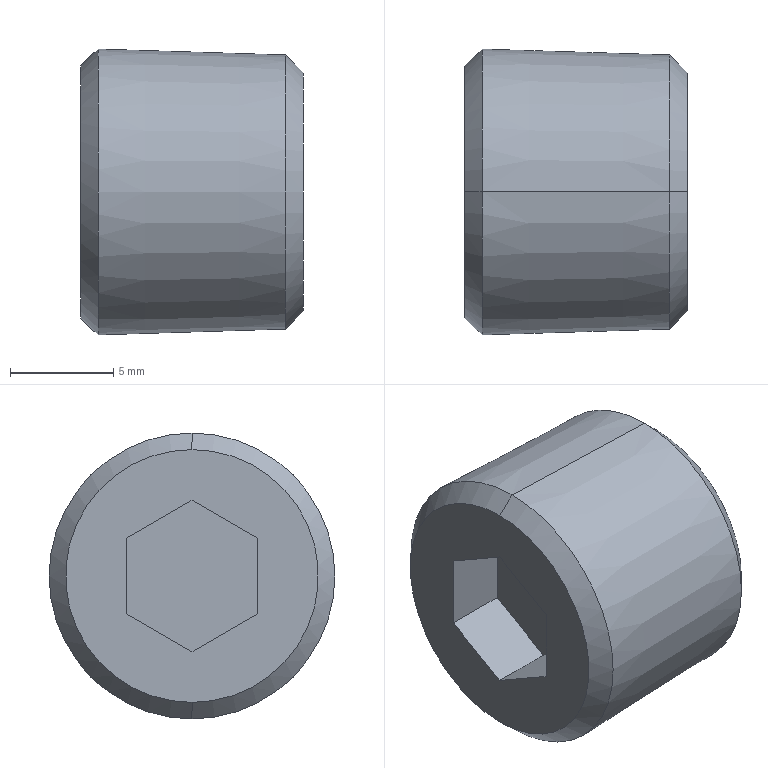Part | STEP file | AC40-04-KSTV-38JNR_AC3009A Plug | 1 solid | 15 faces | box 10.8 x 13.845 x 13.845 mm | volume 1426 mm3 | plane 9 | cone 6
STEP:
#1=CARTESIAN_POINT('',(0.,0.,0.));
#2=DIRECTION('',(0.,0.,1.));
#3=DIRECTION('',(1.,0.,0.));
#4=AXIS2_PLACEMENT_3D('',#1,#2,#3);
#5=CARTESIAN_POINT('',(0.,0.,6.124));
#6=VERTEX_POINT('',#5);
#7=CARTESIAN_POINT('',(0.,0.,-6.124));
#8=VERTEX_POINT('',#7);
#9=CARTESIAN_POINT('',(0.,0.,0.));
#10=DIRECTION('',(-1.,0.,0.));
#11=DIRECTION('',(0.,0.,-1.));
#12=AXIS2_PLACEMENT_3D('',#9,#10,#11);
#13=CIRCLE('',#12,6.124);
#14=CARTESIAN_POINT('',(0.,0.,0.));
#15=DIRECTION('',(1.,0.,0.));
#16=DIRECTION('',(0.,0.,-1.));
#17=AXIS2_PLACEMENT_3D('',#14,#15,#16);
#18=CONICAL_SURFACE('',#17,6.124,0.7543);
#19=CARTESIAN_POINT('',(6.283,0.));
#20=DIRECTION('',(-1.,0.));
#21=VECTOR('',#20,1.);
#22=LINE('',#19,#21);
#23=(GEOMETRIC_REPRESENTATION_CONTEXT(2)PARAMETRIC_REPRESENTATION_CONTEXT()REPRESENTATION_CONTEXT('',''));
#24=DEFINITIONAL_REPRESENTATION('',(#22),#23);
#25=PCURVE('',#18,#24);
#26=CARTESIAN_POINT('',(0.,0.,0.));
#27=DIRECTION('',(1.,0.,0.));
#28=DIRECTION('',(0.,0.,-1.));
#29=AXIS2_PLACEMENT_3D('',#26,#27,#28);
#30=PLANE('',#29);
#31=CARTESIAN_POINT('',(6.124,0.));
#32=CARTESIAN_POINT('',(6.124,-10.608));
#33=CARTESIAN_POINT('',(-3.062,-5.304));
#34=CARTESIAN_POINT('',(-12.249,0.));
#35=CARTESIAN_POINT('',(-3.062,5.304));
#36=CARTESIAN_POINT('',(6.124,10.608));
#37=CARTESIAN_POINT('',(6.124,0.));
#38=(BOUNDED_CURVE()B_SPLINE_CURVE(2,(#31,#32,#33,#34,#35,#36,#37),.UNSPECIFIED.,.T.,.F.)B_SPLINE_CURVE_WITH_KNOTS((1,2,2,2,2,1),(-2.094,0.,2.094,4.189,6.283,8.378),.UNSPECIFIED.)CURVE()GEOMETRIC_REPRESENTATION_ITEM()RATIONAL_B_SPLINE_CURVE((1.,0.5,1.,0.5,1.,0.5,1.))REPRESENTATION_ITEM(''));
#39=(GEOMETRIC_REPRESENTATION_CONTEXT(2)PARAMETRIC_REPRESENTATION_CONTEXT()REPRESENTATION_CONTEXT('',''));
#40=DEFINITIONAL_REPRESENTATION('',(#38),#39);
#41=PCURVE('',#30,#40);
#42=SURFACE_CURVE('',#13,(#25,#41),.PCURVE_S1.);
#43=EDGE_CURVE('',#6,#8,#42,.T.);
#44=ORIENTED_EDGE('',*,*,#43,.F.);
#45=CARTESIAN_POINT('',(0.8496,0.,6.923));
#46=VERTEX_POINT('',#45);
#47=CARTESIAN_POINT('',(0.,0.,6.124));
#48=DIRECTION('',(0.7288,0.,0.6848));
#49=VECTOR('',#48,1.);
#50=LINE('',#47,#49);
#51=CARTESIAN_POINT('',(3.142,0.));
#52=DIRECTION('',(0.,1.));
#53=VECTOR('',#52,1.);
#54=LINE('',#51,#53);
#55=(GEOMETRIC_REPRESENTATION_CONTEXT(2)PARAMETRIC_REPRESENTATION_CONTEXT()REPRESENTATION_CONTEXT('',''));
#56=DEFINITIONAL_REPRESENTATION('',(#54),#55);
#57=PCURVE('',#18,#56);
#58=CARTESIAN_POINT('',(0.,0.,0.));
#59=DIRECTION('',(1.,0.,0.));
#60=DIRECTION('',(0.,0.,-1.));
#61=AXIS2_PLACEMENT_3D('',#58,#59,#60);
#62=CONICAL_SURFACE('',#61,6.124,0.7543);
#63=CARTESIAN_POINT('',(3.142,0.));
#64=DIRECTION('',(0.,1.));
#65=VECTOR('',#64,1.);
#66=LINE('',#63,#65);
#67=(GEOMETRIC_REPRESENTATION_CONTEXT(2)PARAMETRIC_REPRESENTATION_CONTEXT()REPRESENTATION_CONTEXT('',''));
#68=DEFINITIONAL_REPRESENTATION('',(#66),#67);
#69=PCURVE('',#62,#68);
#70=SURFACE_CURVE('',#50,(#57,#69),.PCURVE_S1.);
#71=EDGE_CURVE('',#6,#46,#70,.T.);
#72=ORIENTED_EDGE('',*,*,#71,.T.);
#73=CARTESIAN_POINT('',(0.8496,0.,-6.923));
#74=VERTEX_POINT('',#73);
#75=CARTESIAN_POINT('',(0.8496,0.,0.));
#76=DIRECTION('',(1.,0.,0.));
#77=DIRECTION('',(0.,0.,-1.));
#78=AXIS2_PLACEMENT_3D('',#75,#76,#77);
#79=CIRCLE('',#78,6.923);
#80=CARTESIAN_POINT('',(0.,0.8496));
#81=DIRECTION('',(1.,0.));
#82=VECTOR('',#81,1.);
#83=LINE('',#80,#82);
#84=(GEOMETRIC_REPRESENTATION_CONTEXT(2)PARAMETRIC_REPRESENTATION_CONTEXT()REPRESENTATION_CONTEXT('',''));
#85=DEFINITIONAL_REPRESENTATION('',(#83),#84);
#86=PCURVE('',#18,#85);
#87=CARTESIAN_POINT('',(10.8,0.,0.));
#88=DIRECTION('',(-1.,0.,0.));
#89=DIRECTION('',(0.,0.,1.));
#90=AXIS2_PLACEMENT_3D('',#87,#88,#89);
#91=CONICAL_SURFACE('',#90,6.613,0.03112);
#92=CARTESIAN_POINT('',(3.142,9.95));
#93=DIRECTION('',(-1.,0.));
#94=VECTOR('',#93,1.);
#95=LINE('',#92,#94);
#96=(GEOMETRIC_REPRESENTATION_CONTEXT(2)PARAMETRIC_REPRESENTATION_CONTEXT()REPRESENTATION_CONTEXT('',''));
#97=DEFINITIONAL_REPRESENTATION('',(#95),#96);
#98=PCURVE('',#91,#97);
#99=SURFACE_CURVE('',#79,(#86,#98),.PCURVE_S1.);
#100=EDGE_CURVE('',#74,#46,#99,.T.);
#101=ORIENTED_EDGE('',*,*,#100,.F.);
#102=CARTESIAN_POINT('',(0.,0.,-6.124));
#103=DIRECTION('',(0.7288,0.,-0.6848));
#104=VECTOR('',#103,1.);
#105=LINE('',#102,#104);
#106=CARTESIAN_POINT('',(0.,0.));
#107=DIRECTION('',(0.,1.));
#108=VECTOR('',#107,1.);
#109=LINE('',#106,#108);
#110=(GEOMETRIC_REPRESENTATION_CONTEXT(2)PARAMETRIC_REPRESENTATION_CONTEXT()REPRESENTATION_CONTEXT('',''));
#111=DEFINITIONAL_REPRESENTATION('',(#109),#110);
#112=PCURVE('',#18,#111);
#113=CARTESIAN_POINT('',(6.283,0.));
#114=DIRECTION('',(0.,1.));
#115=VECTOR('',#114,1.);
#116=LINE('',#113,#115);
#117=(GEOMETRIC_REPRESENTATION_CONTEXT(2)PARAMETRIC_REPRESENTATION_CONTEXT()REPRESENTATION_CONTEXT('',''));
#118=DEFINITIONAL_REPRESENTATION('',(#116),#117);
#119=PCURVE('',#62,#118);
#120=SURFACE_CURVE('',#105,(#112,#119),.PCURVE_S1.);
#121=EDGE_CURVE('',#8,#74,#120,.T.);
#122=ORIENTED_EDGE('',*,*,#121,.F.);
#123=EDGE_LOOP('',(#44,#72,#101,#122));
#124=FACE_BOUND('',#123,.T.);
#125=ADVANCED_FACE('',(#124),#18,.T.);
#126=CARTESIAN_POINT('',(10.8,0.,-5.763));
#127=VERTEX_POINT('',#126);
#128=CARTESIAN_POINT('',(10.8,0.,5.763));
#129=VERTEX_POINT('',#128);
#130=CARTESIAN_POINT('',(10.8,0.,0.));
#131=DIRECTION('',(1.,0.,0.));
#132=DIRECTION('',(0.,0.,1.));
#133=AXIS2_PLACEMENT_3D('',#130,#131,#132);
#134=CIRCLE('',#133,5.763);
#135=CARTESIAN_POINT('',(9.923,0.,0.));
#136=DIRECTION('',(-1.,0.,0.));
#137=DIRECTION('',(0.,0.,1.));
#138=AXIS2_PLACEMENT_3D('',#135,#136,#137);
#139=CONICAL_SURFACE('',#138,6.64,0.7854);
#140=CARTESIAN_POINT('',(6.283,-0.8773));
#141=DIRECTION('',(-1.,0.));
#142=VECTOR('',#141,1.);
#143=LINE('',#140,#142);
#144=(GEOMETRIC_REPRESENTATION_CONTEXT(2)PARAMETRIC_REPRESENTATION_CONTEXT()REPRESENTATION_CONTEXT('',''));
#145=DEFINITIONAL_REPRESENTATION('',(#143),#144);
#146=PCURVE('',#139,#145);
#147=CARTESIAN_POINT('',(10.8,6.613,0.));
#148=DIRECTION('',(-1.,0.,0.));
#149=DIRECTION('',(0.,0.,1.));
#150=AXIS2_PLACEMENT_3D('',#147,#148,#149);
#151=PLANE('',#150);
#152=CARTESIAN_POINT('',(5.763,-6.613));
#153=CARTESIAN_POINT('',(5.763,-16.595));
#154=CARTESIAN_POINT('',(-2.881,-11.604));
#155=CARTESIAN_POINT('',(-11.526,-6.613));
#156=CARTESIAN_POINT('',(-2.881,-1.622));
#157=CARTESIAN_POINT('',(5.763,3.369));
#158=CARTESIAN_POINT('',(5.763,-6.613));
#159=(BOUNDED_CURVE()B_SPLINE_CURVE(2,(#152,#153,#154,#155,#156,#157,#158),.UNSPECIFIED.,.T.,.F.)B_SPLINE_CURVE_WITH_KNOTS((1,2,2,2,2,1),(-2.094,0.,2.094,4.189,6.283,8.378),.UNSPECIFIED.)CURVE()GEOMETRIC_REPRESENTATION_ITEM()RATIONAL_B_SPLINE_CURVE((1.,0.5,1.,0.5,1.,0.5,1.))REPRESENTATION_ITEM(''));
#160=(GEOMETRIC_REPRESENTATION_CONTEXT(2)PARAMETRIC_REPRESENTATION_CONTEXT()REPRESENTATION_CONTEXT('',''));
#161=DEFINITIONAL_REPRESENTATION('',(#159),#160);
#162=PCURVE('',#151,#161);
#163=SURFACE_CURVE('',#134,(#146,#162),.PCURVE_S1.);
#164=EDGE_CURVE('',#127,#129,#163,.T.);
#165=ORIENTED_EDGE('',*,*,#164,.F.);
#166=CARTESIAN_POINT('',(9.923,0.,-6.64));
#167=VERTEX_POINT('',#166);
#168=CARTESIAN_POINT('',(9.923,0.,-6.64));
#169=DIRECTION('',(-0.7071,0.,-0.7071));
#170=VECTOR('',#169,1.);
#171=LINE('',#168,#170);
#172=CARTESIAN_POINT('',(3.142,0.));
#173=DIRECTION('',(0.,1.));
#174=VECTOR('',#173,1.);
#175=LINE('',#172,#174);
#176=(GEOMETRIC_REPRESENTATION_CONTEXT(2)PARAMETRIC_REPRESENTATION_CONTEXT()REPRESENTATION_CONTEXT('',''));
#177=DEFINITIONAL_REPRESENTATION('',(#175),#176);
#178=PCURVE('',#139,#177);
#179=CARTESIAN_POINT('',(9.923,0.,0.));
#180=DIRECTION('',(-1.,0.,0.));
#181=DIRECTION('',(0.,0.,1.));
#182=AXIS2_PLACEMENT_3D('',#179,#180,#181);
#183=CONICAL_SURFACE('',#182,6.64,0.7854);
#184=CARTESIAN_POINT('',(3.142,0.));
#185=DIRECTION('',(0.,1.));
#186=VECTOR('',#185,1.);
#187=LINE('',#184,#186);
#188=(GEOMETRIC_REPRESENTATION_CONTEXT(2)PARAMETRIC_REPRESENTATION_CONTEXT()REPRESENTATION_CONTEXT('',''));
#189=DEFINITIONAL_REPRESENTATION('',(#187),#188);
#190=PCURVE('',#183,#189);
#191=SURFACE_CURVE('',#171,(#178,#190),.PCURVE_S1.);
#192=EDGE_CURVE('',#127,#167,#191,.T.);
#193=ORIENTED_EDGE('',*,*,#192,.T.);
#194=CARTESIAN_POINT('',(9.923,0.,6.64));
#195=VERTEX_POINT('',#194);
#196=CARTESIAN_POINT('',(9.923,0.,0.));
#197=DIRECTION('',(-1.,0.,0.));
#198=DIRECTION('',(0.,0.,-1.));
#199=AXIS2_PLACEMENT_3D('',#196,#197,#198);
#200=CIRCLE('',#199,6.64);
#201=CARTESIAN_POINT('',(-3.142,0.));
#202=DIRECTION('',(1.,0.));
#203=VECTOR('',#202,1.);
#204=LINE('',#201,#203);
#205=(GEOMETRIC_REPRESENTATION_CONTEXT(2)PARAMETRIC_REPRESENTATION_CONTEXT()REPRESENTATION_CONTEXT('',''));
#206=DEFINITIONAL_REPRESENTATION('',(#204),#205);
#207=PCURVE('',#139,#206);
#208=CARTESIAN_POINT('',(-3.142,0.8773));
#209=DIRECTION('',(1.,0.));
#210=VECTOR('',#209,1.);
#211=LINE('',#208,#210);
#212=(GEOMETRIC_REPRESENTATION_CONTEXT(2)PARAMETRIC_REPRESENTATION_CONTEXT()REPRESENTATION_CONTEXT('',''));
#213=DEFINITIONAL_REPRESENTATION('',(#211),#212);
#214=PCURVE('',#91,#213);
#215=SURFACE_CURVE('',#200,(#207,#214),.PCURVE_S1.);
#216=EDGE_CURVE('',#195,#167,#215,.T.);
#217=ORIENTED_EDGE('',*,*,#216,.F.);
#218=CARTESIAN_POINT('',(9.923,0.,6.64));
#219=DIRECTION('',(-0.7071,0.,0.7071));
#220=VECTOR('',#219,1.);
#221=LINE('',#218,#220);
#222=CARTESIAN_POINT('',(0.,0.));
#223=DIRECTION('',(0.,1.));
#224=VECTOR('',#223,1.);
#225=LINE('',#222,#224);
#226=(GEOMETRIC_REPRESENTATION_CONTEXT(2)PARAMETRIC_REPRESENTATION_CONTEXT()REPRESENTATION_CONTEXT('',''));
#227=DEFINITIONAL_REPRESENTATION('',(#225),#226);
#228=PCURVE('',#139,#227);
#229=CARTESIAN_POINT('',(6.283,0.));
#230=DIRECTION('',(0.,1.));
#231=VECTOR('',#230,1.);
#232=LINE('',#229,#231);
#233=(GEOMETRIC_REPRESENTATION_CONTEXT(2)PARAMETRIC_REPRESENTATION_CONTEXT()REPRESENTATION_CONTEXT('',''));
#234=DEFINITIONAL_REPRESENTATION('',(#232),#233);
#235=PCURVE('',#183,#234);
#236=SURFACE_CURVE('',#221,(#228,#235),.PCURVE_S1.);
#237=EDGE_CURVE('',#129,#195,#236,.T.);
#238=ORIENTED_EDGE('',*,*,#237,.F.);
#239=EDGE_LOOP('',(#165,#193,#217,#238));
#240=FACE_BOUND('',#239,.T.);
#241=ADVANCED_FACE('',(#240),#139,.T.);
#242=ORIENTED_EDGE('',*,*,#216,.T.);
#243=CARTESIAN_POINT('',(10.8,0.,-6.613));
#244=DIRECTION('',(-0.9995,0.,-0.03111));
#245=VECTOR('',#244,1.);
#246=LINE('',#243,#245);
#247=CARTESIAN_POINT('',(3.142,0.));
#248=DIRECTION('',(0.,1.));
#249=VECTOR('',#248,1.);
#250=LINE('',#247,#249);
#251=(GEOMETRIC_REPRESENTATION_CONTEXT(2)PARAMETRIC_REPRESENTATION_CONTEXT()REPRESENTATION_CONTEXT('',''));
#252=DEFINITIONAL_REPRESENTATION('',(#250),#251);
#253=PCURVE('',#91,#252);
#254=CARTESIAN_POINT('',(10.8,0.,0.));
#255=DIRECTION('',(-1.,0.,0.));
#256=DIRECTION('',(0.,0.,1.));
#257=AXIS2_PLACEMENT_3D('',#254,#255,#256);
#258=CONICAL_SURFACE('',#257,6.613,0.03112);
#259=CARTESIAN_POINT('',(3.142,0.));
#260=DIRECTION('',(0.,1.));
#261=VECTOR('',#260,1.);
#262=LINE('',#259,#261);
#263=(GEOMETRIC_REPRESENTATION_CONTEXT(2)PARAMETRIC_REPRESENTATION_CONTEXT()REPRESENTATION_CONTEXT('',''));
#264=DEFINITIONAL_REPRESENTATION('',(#262),#263);
#265=PCURVE('',#258,#264);
#266=SURFACE_CURVE('',#246,(#253,#265),.PCURVE_S1.);
#267=EDGE_CURVE('',#167,#74,#266,.T.);
#268=ORIENTED_EDGE('',*,*,#267,.T.);
#269=ORIENTED_EDGE('',*,*,#100,.T.);
#270=CARTESIAN_POINT('',(10.8,0.,6.613));
#271=DIRECTION('',(-0.9995,0.,0.03111));
#272=VECTOR('',#271,1.);
#273=LINE('',#270,#272);
#274=CARTESIAN_POINT('',(0.,0.));
#275=DIRECTION('',(0.,1.));
#276=VECTOR('',#275,1.);
#277=LINE('',#274,#276);
#278=(GEOMETRIC_REPRESENTATION_CONTEXT(2)PARAMETRIC_REPRESENTATION_CONTEXT()REPRESENTATION_CONTEXT('',''));
#279=DEFINITIONAL_REPRESENTATION('',(#277),#278);
#280=PCURVE('',#91,#279);
#281=CARTESIAN_POINT('',(6.283,0.));
#282=DIRECTION('',(0.,1.));
#283=VECTOR('',#282,1.);
#284=LINE('',#281,#283);
#285=(GEOMETRIC_REPRESENTATION_CONTEXT(2)PARAMETRIC_REPRESENTATION_CONTEXT()REPRESENTATION_CONTEXT('',''));
#286=DEFINITIONAL_REPRESENTATION('',(#284),#285);
#287=PCURVE('',#258,#286);
#288=SURFACE_CURVE('',#273,(#280,#287),.PCURVE_S1.);
#289=EDGE_CURVE('',#195,#46,#288,.T.);
#290=ORIENTED_EDGE('',*,*,#289,.F.);
#291=EDGE_LOOP('',(#242,#268,#269,#290));
#292=FACE_BOUND('',#291,.T.);
#293=ADVANCED_FACE('',(#292),#91,.T.);
#294=CARTESIAN_POINT('',(10.8,0.,0.));
#295=DIRECTION('',(1.,0.,0.));
#296=DIRECTION('',(0.,0.,1.));
#297=AXIS2_PLACEMENT_3D('',#294,#295,#296);
#298=CIRCLE('',#297,5.763);
#299=CARTESIAN_POINT('',(5.763,-6.613));
#300=CARTESIAN_POINT('',(5.763,-16.595));
#301=CARTESIAN_POINT('',(-2.881,-11.604));
#302=CARTESIAN_POINT('',(-11.526,-6.613));
#303=CARTESIAN_POINT('',(-2.881,-1.622));
#304=CARTESIAN_POINT('',(5.763,3.369));
#305=CARTESIAN_POINT('',(5.763,-6.613));
#306=(BOUNDED_CURVE()B_SPLINE_CURVE(2,(#299,#300,#301,#302,#303,#304,#305),.UNSPECIFIED.,.T.,.F.)B_SPLINE_CURVE_WITH_KNOTS((1,2,2,2,2,1),(-2.094,0.,2.094,4.189,6.283,8.378),.UNSPECIFIED.)CURVE()GEOMETRIC_REPRESENTATION_ITEM()RATIONAL_B_SPLINE_CURVE((1.,0.5,1.,0.5,1.,0.5,1.))REPRESENTATION_ITEM(''));
#307=(GEOMETRIC_REPRESENTATION_CONTEXT(2)PARAMETRIC_REPRESENTATION_CONTEXT()REPRESENTATION_CONTEXT('',''));
#308=DEFINITIONAL_REPRESENTATION('',(#306),#307);
#309=PCURVE('',#151,#308);
#310=CARTESIAN_POINT('',(6.283,-0.8773));
#311=DIRECTION('',(-1.,0.));
#312=VECTOR('',#311,1.);
#313=LINE('',#310,#312);
#314=(GEOMETRIC_REPRESENTATION_CONTEXT(2)PARAMETRIC_REPRESENTATION_CONTEXT()REPRESENTATION_CONTEXT('',''));
#315=DEFINITIONAL_REPRESENTATION('',(#313),#314);
#316=PCURVE('',#183,#315);
#317=SURFACE_CURVE('',#298,(#309,#316),.PCURVE_S1.);
#318=EDGE_CURVE('',#129,#127,#317,.T.);
#319=ORIENTED_EDGE('',*,*,#318,.T.);
#320=ORIENTED_EDGE('',*,*,#164,.T.);
#321=EDGE_LOOP('',(#319,#320));
#322=FACE_BOUND('',#321,.T.);
#323=ADVANCED_FACE('',(#322),#151,.F.);
#324=ORIENTED_EDGE('',*,*,#267,.F.);
#325=CARTESIAN_POINT('',(9.923,0.,0.));
#326=DIRECTION('',(-1.,0.,0.));
#327=DIRECTION('',(0.,0.,-1.));
#328=AXIS2_PLACEMENT_3D('',#325,#326,#327);
#329=CIRCLE('',#328,6.64);
#330=CARTESIAN_POINT('',(3.142,0.8773));
#331=DIRECTION('',(1.,0.));
#332=VECTOR('',#331,1.);
#333=LINE('',#330,#332);
#334=(GEOMETRIC_REPRESENTATION_CONTEXT(2)PARAMETRIC_REPRESENTATION_CONTEXT()REPRESENTATION_CONTEXT('',''));
#335=DEFINITIONAL_REPRESENTATION('',(#333),#334);
#336=PCURVE('',#258,#335);
#337=CARTESIAN_POINT('',(3.142,0.));
#338=DIRECTION('',(1.,0.));
#339=VECTOR('',#338,1.);
#340=LINE('',#337,#339);
#341=(GEOMETRIC_REPRESENTATION_CONTEXT(2)PARAMETRIC_REPRESENTATION_CONTEXT()REPRESENTATION_CONTEXT('',''));
#342=DEFINITIONAL_REPRESENTATION('',(#340),#341);
#343=PCURVE('',#183,#342);
#344=SURFACE_CURVE('',#329,(#336,#343),.PCURVE_S1.);
#345=EDGE_CURVE('',#167,#195,#344,.T.);
#346=ORIENTED_EDGE('',*,*,#345,.T.);
#347=ORIENTED_EDGE('',*,*,#289,.T.);
#348=CARTESIAN_POINT('',(0.8496,0.,0.));
#349=DIRECTION('',(1.,0.,0.));
#350=DIRECTION('',(0.,0.,-1.));
#351=AXIS2_PLACEMENT_3D('',#348,#349,#350);
#352=CIRCLE('',#351,6.923);
#353=CARTESIAN_POINT('',(9.425,9.95));
#354=DIRECTION('',(-1.,0.));
#355=VECTOR('',#354,1.);
#356=LINE('',#353,#355);
#357=(GEOMETRIC_REPRESENTATION_CONTEXT(2)PARAMETRIC_REPRESENTATION_CONTEXT()REPRESENTATION_CONTEXT('',''));
#358=DEFINITIONAL_REPRESENTATION('',(#356),#357);
#359=PCURVE('',#258,#358);
#360=CARTESIAN_POINT('',(0.,0.8496));
#361=DIRECTION('',(1.,0.));
#362=VECTOR('',#361,1.);
#363=LINE('',#360,#362);
#364=(GEOMETRIC_REPRESENTATION_CONTEXT(2)PARAMETRIC_REPRESENTATION_CONTEXT()REPRESENTATION_CONTEXT('',''));
#365=DEFINITIONAL_REPRESENTATION('',(#363),#364);
#366=PCURVE('',#62,#365);
#367=SURFACE_CURVE('',#352,(#359,#366),.PCURVE_S1.);
#368=EDGE_CURVE('',#46,#74,#367,.T.);
#369=ORIENTED_EDGE('',*,*,#368,.T.);
#370=EDGE_LOOP('',(#324,#346,#347,#369));
#371=FACE_BOUND('',#370,.T.);
#372=ADVANCED_FACE('',(#371),#258,.T.);
#373=CARTESIAN_POINT('',(0.,0.,3.666));
#374=VERTEX_POINT('',#373);
#375=CARTESIAN_POINT('',(0.,3.175,1.833));
#376=VERTEX_POINT('',#375);
#377=CARTESIAN_POINT('',(0.,0.,3.666));
#378=DIRECTION('',(0.,0.866,-0.5));
#379=VECTOR('',#378,1.);
#380=LINE('',#377,#379);
#381=CARTESIAN_POINT('',(-3.666,0.));
#382=DIRECTION('',(0.5,0.866));
#383=VECTOR('',#382,1.);
#384=LINE('',#381,#383);
#385=(GEOMETRIC_REPRESENTATION_CONTEXT(2)PARAMETRIC_REPRESENTATION_CONTEXT()REPRESENTATION_CONTEXT('',''));
#386=DEFINITIONAL_REPRESENTATION('',(#384),#385);
#387=PCURVE('',#30,#386);
#388=CARTESIAN_POINT('',(3.,0.,3.666));
#389=DIRECTION('',(0.,0.5,0.866));
#390=DIRECTION('',(0.,-0.866,0.5));
#391=AXIS2_PLACEMENT_3D('',#388,#389,#390);
#392=PLANE('',#391);
#393=CARTESIAN_POINT('',(0.,-3.));
#394=DIRECTION('',(-1.,0.));
#395=VECTOR('',#394,1.);
#396=LINE('',#393,#395);
#397=(GEOMETRIC_REPRESENTATION_CONTEXT(2)PARAMETRIC_REPRESENTATION_CONTEXT()REPRESENTATION_CONTEXT('',''));
#398=DEFINITIONAL_REPRESENTATION('',(#396),#397);
#399=PCURVE('',#392,#398);
#400=SURFACE_CURVE('',#380,(#387,#399),.PCURVE_S1.);
#401=EDGE_CURVE('',#374,#376,#400,.T.);
#402=ORIENTED_EDGE('',*,*,#401,.F.);
#403=CARTESIAN_POINT('',(0.,-3.175,1.833));
#404=VERTEX_POINT('',#403);
#405=CARTESIAN_POINT('',(0.,-3.175,1.833));
#406=DIRECTION('',(0.,0.866,0.5));
#407=VECTOR('',#406,1.);
#408=LINE('',#405,#407);
#409=CARTESIAN_POINT('',(-1.833,-3.175));
#410=DIRECTION('',(-0.5,0.866));
#411=VECTOR('',#410,1.);
#412=LINE('',#409,#411);
#413=(GEOMETRIC_REPRESENTATION_CONTEXT(2)PARAMETRIC_REPRESENTATION_CONTEXT()REPRESENTATION_CONTEXT('',''));
#414=DEFINITIONAL_REPRESENTATION('',(#412),#413);
#415=PCURVE('',#30,#414);
#416=CARTESIAN_POINT('',(3.,-3.175,1.833));
#417=DIRECTION('',(0.,-0.5,0.866));
#418=DIRECTION('',(0.,-0.866,-0.5));
#419=AXIS2_PLACEMENT_3D('',#416,#417,#418);
#420=PLANE('',#419);
#421=CARTESIAN_POINT('',(0.,-3.));
#422=DIRECTION('',(-1.,0.));
#423=VECTOR('',#422,1.);
#424=LINE('',#421,#423);
#425=(GEOMETRIC_REPRESENTATION_CONTEXT(2)PARAMETRIC_REPRESENTATION_CONTEXT()REPRESENTATION_CONTEXT('',''));
#426=DEFINITIONAL_REPRESENTATION('',(#424),#425);
#427=PCURVE('',#420,#426);
#428=SURFACE_CURVE('',#408,(#415,#427),.PCURVE_S1.);
#429=EDGE_CURVE('',#404,#374,#428,.T.);
#430=ORIENTED_EDGE('',*,*,#429,.F.);
#431=CARTESIAN_POINT('',(0.,-3.175,-1.833));
#432=VERTEX_POINT('',#431);
#433=CARTESIAN_POINT('',(0.,-3.175,-1.833));
#434=DIRECTION('',(0.,0.,1.));
#435=VECTOR('',#434,1.);
#436=LINE('',#433,#435);
#437=CARTESIAN_POINT('',(1.833,-3.175));
#438=DIRECTION('',(-1.,0.));
#439=VECTOR('',#438,1.);
#440=LINE('',#437,#439);
#441=(GEOMETRIC_REPRESENTATION_CONTEXT(2)PARAMETRIC_REPRESENTATION_CONTEXT()REPRESENTATION_CONTEXT('',''));
#442=DEFINITIONAL_REPRESENTATION('',(#440),#441);
#443=PCURVE('',#30,#442);
#444=CARTESIAN_POINT('',(3.,-3.175,-1.833));
#445=DIRECTION('',(0.,-1.,0.));
#446=DIRECTION('',(0.,0.,-1.));
#447=AXIS2_PLACEMENT_3D('',#444,#445,#446);
#448=PLANE('',#447);
#449=CARTESIAN_POINT('',(0.,-3.));
#450=DIRECTION('',(-1.,0.));
#451=VECTOR('',#450,1.);
#452=LINE('',#449,#451);
#453=(GEOMETRIC_REPRESENTATION_CONTEXT(2)PARAMETRIC_REPRESENTATION_CONTEXT()REPRESENTATION_CONTEXT('',''));
#454=DEFINITIONAL_REPRESENTATION('',(#452),#453);
#455=PCURVE('',#448,#454);
#456=SURFACE_CURVE('',#436,(#443,#455),.PCURVE_S1.);
#457=EDGE_CURVE('',#432,#404,#456,.T.);
#458=ORIENTED_EDGE('',*,*,#457,.F.);
#459=CARTESIAN_POINT('',(0.,0.,-3.666));
#460=VERTEX_POINT('',#459);
#461=CARTESIAN_POINT('',(0.,0.,-3.666));
#462=DIRECTION('',(0.,-0.866,0.5));
#463=VECTOR('',#462,1.);
#464=LINE('',#461,#463);
#465=CARTESIAN_POINT('',(3.666,0.));
#466=DIRECTION('',(-0.5,-0.866));
#467=VECTOR('',#466,1.);
#468=LINE('',#465,#467);
#469=(GEOMETRIC_REPRESENTATION_CONTEXT(2)PARAMETRIC_REPRESENTATION_CONTEXT()REPRESENTATION_CONTEXT('',''));
#470=DEFINITIONAL_REPRESENTATION('',(#468),#469);
#471=PCURVE('',#30,#470);
#472=CARTESIAN_POINT('',(3.,0.,-3.666));
#473=DIRECTION('',(0.,-0.5,-0.866));
#474=DIRECTION('',(0.,0.866,-0.5));
#475=AXIS2_PLACEMENT_3D('',#472,#473,#474);
#476=PLANE('',#475);
#477=CARTESIAN_POINT('',(0.,-3.));
#478=DIRECTION('',(-1.,0.));
#479=VECTOR('',#478,1.);
#480=LINE('',#477,#479);
#481=(GEOMETRIC_REPRESENTATION_CONTEXT(2)PARAMETRIC_REPRESENTATION_CONTEXT()REPRESENTATION_CONTEXT('',''));
#482=DEFINITIONAL_REPRESENTATION('',(#480),#481);
#483=PCURVE('',#476,#482);
#484=SURFACE_CURVE('',#464,(#471,#483),.PCURVE_S1.);
#485=EDGE_CURVE('',#460,#432,#484,.T.);
#486=ORIENTED_EDGE('',*,*,#485,.F.);
#487=CARTESIAN_POINT('',(0.,3.175,-1.833));
#488=VERTEX_POINT('',#487);
#489=CARTESIAN_POINT('',(0.,3.175,-1.833));
#490=DIRECTION('',(0.,-0.866,-0.5));
#491=VECTOR('',#490,1.);
#492=LINE('',#489,#491);
#493=CARTESIAN_POINT('',(1.833,3.175));
#494=DIRECTION('',(0.5,-0.866));
#495=VECTOR('',#494,1.);
#496=LINE('',#493,#495);
#497=(GEOMETRIC_REPRESENTATION_CONTEXT(2)PARAMETRIC_REPRESENTATION_CONTEXT()REPRESENTATION_CONTEXT('',''));
#498=DEFINITIONAL_REPRESENTATION('',(#496),#497);
#499=PCURVE('',#30,#498);
#500=CARTESIAN_POINT('',(3.,3.175,-1.833));
#501=DIRECTION('',(0.,0.5,-0.866));
#502=DIRECTION('',(0.,0.866,0.5));
#503=AXIS2_PLACEMENT_3D('',#500,#501,#502);
#504=PLANE('',#503);
#505=CARTESIAN_POINT('',(0.,-3.));
#506=DIRECTION('',(-1.,0.));
#507=VECTOR('',#506,1.);
#508=LINE('',#505,#507);
#509=(GEOMETRIC_REPRESENTATION_CONTEXT(2)PARAMETRIC_REPRESENTATION_CONTEXT()REPRESENTATION_CONTEXT('',''));
#510=DEFINITIONAL_REPRESENTATION('',(#508),#509);
#511=PCURVE('',#504,#510);
#512=SURFACE_CURVE('',#492,(#499,#511),.PCURVE_S1.);
#513=EDGE_CURVE('',#488,#460,#512,.T.);
#514=ORIENTED_EDGE('',*,*,#513,.F.);
#515=CARTESIAN_POINT('',(0.,3.175,1.833));
#516=DIRECTION('',(0.,0.,-1.));
#517=VECTOR('',#516,1.);
#518=LINE('',#515,#517);
#519=CARTESIAN_POINT('',(-1.833,3.175));
#520=DIRECTION('',(1.,0.));
#521=VECTOR('',#520,1.);
#522=LINE('',#519,#521);
#523=(GEOMETRIC_REPRESENTATION_CONTEXT(2)PARAMETRIC_REPRESENTATION_CONTEXT()REPRESENTATION_CONTEXT('',''));
#524=DEFINITIONAL_REPRESENTATION('',(#522),#523);
#525=PCURVE('',#30,#524);
#526=CARTESIAN_POINT('',(3.,3.175,1.833));
#527=DIRECTION('',(0.,1.,0.));
#528=DIRECTION('',(0.,0.,1.));
#529=AXIS2_PLACEMENT_3D('',#526,#527,#528);
#530=PLANE('',#529);
#531=CARTESIAN_POINT('',(0.,-3.));
#532=DIRECTION('',(-1.,0.));
#533=VECTOR('',#532,1.);
#534=LINE('',#531,#533);
#535=(GEOMETRIC_REPRESENTATION_CONTEXT(2)PARAMETRIC_REPRESENTATION_CONTEXT()REPRESENTATION_CONTEXT('',''));
#536=DEFINITIONAL_REPRESENTATION('',(#534),#535);
#537=PCURVE('',#530,#536);
#538=SURFACE_CURVE('',#518,(#525,#537),.PCURVE_S1.);
#539=EDGE_CURVE('',#376,#488,#538,.T.);
#540=ORIENTED_EDGE('',*,*,#539,.F.);
#541=EDGE_LOOP('',(#402,#430,#458,#486,#514,#540));
#542=FACE_BOUND('',#541,.T.);
#543=CARTESIAN_POINT('',(0.,0.,0.));
#544=DIRECTION('',(-1.,0.,0.));
#545=DIRECTION('',(0.,0.,-1.));
#546=AXIS2_PLACEMENT_3D('',#543,#544,#545);
#547=CIRCLE('',#546,6.124);
#548=CARTESIAN_POINT('',(6.124,0.));
#549=CARTESIAN_POINT('',(6.124,-10.608));
#550=CARTESIAN_POINT('',(-3.062,-5.304));
#551=CARTESIAN_POINT('',(-12.249,0.));
#552=CARTESIAN_POINT('',(-3.062,5.304));
#553=CARTESIAN_POINT('',(6.124,10.608));
#554=CARTESIAN_POINT('',(6.124,0.));
#555=(BOUNDED_CURVE()B_SPLINE_CURVE(2,(#548,#549,#550,#551,#552,#553,#554),.UNSPECIFIED.,.T.,.F.)B_SPLINE_CURVE_WITH_KNOTS((1,2,2,2,2,1),(-2.094,0.,2.094,4.189,6.283,8.378),.UNSPECIFIED.)CURVE()GEOMETRIC_REPRESENTATION_ITEM()RATIONAL_B_SPLINE_CURVE((1.,0.5,1.,0.5,1.,0.5,1.))REPRESENTATION_ITEM(''));
#556=(GEOMETRIC_REPRESENTATION_CONTEXT(2)PARAMETRIC_REPRESENTATION_CONTEXT()REPRESENTATION_CONTEXT('',''));
#557=DEFINITIONAL_REPRESENTATION('',(#555),#556);
#558=PCURVE('',#30,#557);
#559=CARTESIAN_POINT('',(6.283,0.));
#560=DIRECTION('',(-1.,0.));
#561=VECTOR('',#560,1.);
#562=LINE('',#559,#561);
#563=(GEOMETRIC_REPRESENTATION_CONTEXT(2)PARAMETRIC_REPRESENTATION_CONTEXT()REPRESENTATION_CONTEXT('',''));
#564=DEFINITIONAL_REPRESENTATION('',(#562),#563);
#565=PCURVE('',#62,#564);
#566=SURFACE_CURVE('',#547,(#558,#565),.PCURVE_S1.);
#567=EDGE_CURVE('',#8,#6,#566,.T.);
#568=ORIENTED_EDGE('',*,*,#567,.T.);
#569=ORIENTED_EDGE('',*,*,#43,.T.);
#570=EDGE_LOOP('',(#568,#569));
#571=FACE_BOUND('',#570,.T.);
#572=ADVANCED_FACE('',(#542,#571),#30,.F.);
#573=ORIENTED_EDGE('',*,*,#192,.F.);
#574=ORIENTED_EDGE('',*,*,#318,.F.);
#575=ORIENTED_EDGE('',*,*,#237,.T.);
#576=ORIENTED_EDGE('',*,*,#345,.F.);
#577=EDGE_LOOP('',(#573,#574,#575,#576));
#578=FACE_BOUND('',#577,.T.);
#579=ADVANCED_FACE('',(#578),#183,.T.);
#580=ORIENTED_EDGE('',*,*,#71,.F.);
#581=ORIENTED_EDGE('',*,*,#567,.F.);
#582=ORIENTED_EDGE('',*,*,#121,.T.);
#583=ORIENTED_EDGE('',*,*,#368,.F.);
#584=EDGE_LOOP('',(#580,#581,#582,#583));
#585=FACE_BOUND('',#584,.T.);
#586=ADVANCED_FACE('',(#585),#62,.T.);
#587=ORIENTED_EDGE('',*,*,#429,.T.);
#588=CARTESIAN_POINT('',(3.,0.,3.666));
#589=VERTEX_POINT('',#588);
#590=CARTESIAN_POINT('',(3.,0.,3.666));
#591=DIRECTION('',(-1.,0.,0.));
#592=VECTOR('',#591,1.);
#593=LINE('',#590,#592);
#594=CARTESIAN_POINT('',(-3.666,0.));
#595=DIRECTION('',(0.,-1.));
#596=VECTOR('',#595,1.);
#597=LINE('',#594,#596);
#598=(GEOMETRIC_REPRESENTATION_CONTEXT(2)PARAMETRIC_REPRESENTATION_CONTEXT()REPRESENTATION_CONTEXT('',''));
#599=DEFINITIONAL_REPRESENTATION('',(#597),#598);
#600=PCURVE('',#420,#599);
#601=CARTESIAN_POINT('',(0.,0.));
#602=DIRECTION('',(0.,-1.));
#603=VECTOR('',#602,1.);
#604=LINE('',#601,#603);
#605=(GEOMETRIC_REPRESENTATION_CONTEXT(2)PARAMETRIC_REPRESENTATION_CONTEXT()REPRESENTATION_CONTEXT('',''));
#606=DEFINITIONAL_REPRESENTATION('',(#604),#605);
#607=PCURVE('',#392,#606);
#608=SURFACE_CURVE('',#593,(#600,#607),.PCURVE_S1.);
#609=EDGE_CURVE('',#589,#374,#608,.T.);
#610=ORIENTED_EDGE('',*,*,#609,.F.);
#611=CARTESIAN_POINT('',(3.,-3.175,1.833));
#612=VERTEX_POINT('',#611);
#613=CARTESIAN_POINT('',(3.,-3.175,1.833));
#614=DIRECTION('',(0.,0.866,0.5));
#615=VECTOR('',#614,1.);
#616=LINE('',#613,#615);
#617=CARTESIAN_POINT('',(0.,0.));
#618=DIRECTION('',(-1.,0.));
#619=VECTOR('',#618,1.);
#620=LINE('',#617,#619);
#621=(GEOMETRIC_REPRESENTATION_CONTEXT(2)PARAMETRIC_REPRESENTATION_CONTEXT()REPRESENTATION_CONTEXT('',''));
#622=DEFINITIONAL_REPRESENTATION('',(#620),#621);
#623=PCURVE('',#420,#622);
#624=CARTESIAN_POINT('',(3.,3.175,5.499));
#625=DIRECTION('',(-1.,0.,0.));
#626=DIRECTION('',(0.,0.,1.));
#627=AXIS2_PLACEMENT_3D('',#624,#625,#626);
#628=PLANE('',#627);
#629=CARTESIAN_POINT('',(-3.666,-6.35));
#630=DIRECTION('',(0.5,0.866));
#631=VECTOR('',#630,1.);
#632=LINE('',#629,#631);
#633=(GEOMETRIC_REPRESENTATION_CONTEXT(2)PARAMETRIC_REPRESENTATION_CONTEXT()REPRESENTATION_CONTEXT('',''));
#634=DEFINITIONAL_REPRESENTATION('',(#632),#633);
#635=PCURVE('',#628,#634);
#636=SURFACE_CURVE('',#616,(#623,#635),.PCURVE_S1.);
#637=EDGE_CURVE('',#612,#589,#636,.T.);
#638=ORIENTED_EDGE('',*,*,#637,.F.);
#639=CARTESIAN_POINT('',(3.,-3.175,1.833));
#640=DIRECTION('',(-1.,0.,0.));
#641=VECTOR('',#640,1.);
#642=LINE('',#639,#641);
#643=CARTESIAN_POINT('',(0.,0.));
#644=DIRECTION('',(0.,-1.));
#645=VECTOR('',#644,1.);
#646=LINE('',#643,#645);
#647=(GEOMETRIC_REPRESENTATION_CONTEXT(2)PARAMETRIC_REPRESENTATION_CONTEXT()REPRESENTATION_CONTEXT('',''));
#648=DEFINITIONAL_REPRESENTATION('',(#646),#647);
#649=PCURVE('',#420,#648);
#650=CARTESIAN_POINT('',(-3.666,0.));
#651=DIRECTION('',(0.,-1.));
#652=VECTOR('',#651,1.);
#653=LINE('',#650,#652);
#654=(GEOMETRIC_REPRESENTATION_CONTEXT(2)PARAMETRIC_REPRESENTATION_CONTEXT()REPRESENTATION_CONTEXT('',''));
#655=DEFINITIONAL_REPRESENTATION('',(#653),#654);
#656=PCURVE('',#448,#655);
#657=SURFACE_CURVE('',#642,(#649,#656),.PCURVE_S1.);
#658=EDGE_CURVE('',#612,#404,#657,.T.);
#659=ORIENTED_EDGE('',*,*,#658,.T.);
#660=EDGE_LOOP('',(#587,#610,#638,#659));
#661=FACE_BOUND('',#660,.T.);
#662=ADVANCED_FACE('',(#661),#420,.F.);
#663=ORIENTED_EDGE('',*,*,#457,.T.);
#664=ORIENTED_EDGE('',*,*,#658,.F.);
#665=CARTESIAN_POINT('',(3.,-3.175,-1.833));
#666=VERTEX_POINT('',#665);
#667=CARTESIAN_POINT('',(3.,-3.175,-1.833));
#668=DIRECTION('',(0.,0.,1.));
#669=VECTOR('',#668,1.);
#670=LINE('',#667,#669);
#671=CARTESIAN_POINT('',(0.,0.));
#672=DIRECTION('',(-1.,0.));
#673=VECTOR('',#672,1.);
#674=LINE('',#671,#673);
#675=(GEOMETRIC_REPRESENTATION_CONTEXT(2)PARAMETRIC_REPRESENTATION_CONTEXT()REPRESENTATION_CONTEXT('',''));
#676=DEFINITIONAL_REPRESENTATION('',(#674),#675);
#677=PCURVE('',#448,#676);
#678=CARTESIAN_POINT('',(-7.332,-6.35));
#679=DIRECTION('',(1.,0.));
#680=VECTOR('',#679,1.);
#681=LINE('',#678,#680);
#682=(GEOMETRIC_REPRESENTATION_CONTEXT(2)PARAMETRIC_REPRESENTATION_CONTEXT()REPRESENTATION_CONTEXT('',''));
#683=DEFINITIONAL_REPRESENTATION('',(#681),#682);
#684=PCURVE('',#628,#683);
#685=SURFACE_CURVE('',#670,(#677,#684),.PCURVE_S1.);
#686=EDGE_CURVE('',#666,#612,#685,.T.);
#687=ORIENTED_EDGE('',*,*,#686,.F.);
#688=CARTESIAN_POINT('',(3.,-3.175,-1.833));
#689=DIRECTION('',(-1.,0.,0.));
#690=VECTOR('',#689,1.);
#691=LINE('',#688,#690);
#692=CARTESIAN_POINT('',(0.,0.));
#693=DIRECTION('',(0.,-1.));
#694=VECTOR('',#693,1.);
#695=LINE('',#692,#694);
#696=(GEOMETRIC_REPRESENTATION_CONTEXT(2)PARAMETRIC_REPRESENTATION_CONTEXT()REPRESENTATION_CONTEXT('',''));
#697=DEFINITIONAL_REPRESENTATION('',(#695),#696);
#698=PCURVE('',#448,#697);
#699=CARTESIAN_POINT('',(-3.666,0.));
#700=DIRECTION('',(0.,-1.));
#701=VECTOR('',#700,1.);
#702=LINE('',#699,#701);
#703=(GEOMETRIC_REPRESENTATION_CONTEXT(2)PARAMETRIC_REPRESENTATION_CONTEXT()REPRESENTATION_CONTEXT('',''));
#704=DEFINITIONAL_REPRESENTATION('',(#702),#703);
#705=PCURVE('',#476,#704);
#706=SURFACE_CURVE('',#691,(#698,#705),.PCURVE_S1.);
#707=EDGE_CURVE('',#666,#432,#706,.T.);
#708=ORIENTED_EDGE('',*,*,#707,.T.);
#709=EDGE_LOOP('',(#663,#664,#687,#708));
#710=FACE_BOUND('',#709,.T.);
#711=ADVANCED_FACE('',(#710),#448,.F.);
#712=ORIENTED_EDGE('',*,*,#485,.T.);
#713=ORIENTED_EDGE('',*,*,#707,.F.);
#714=CARTESIAN_POINT('',(3.,0.,-3.666));
#715=VERTEX_POINT('',#714);
#716=CARTESIAN_POINT('',(3.,0.,-3.666));
#717=DIRECTION('',(0.,-0.866,0.5));
#718=VECTOR('',#717,1.);
#719=LINE('',#716,#718);
#720=CARTESIAN_POINT('',(0.,0.));
#721=DIRECTION('',(-1.,0.));
#722=VECTOR('',#721,1.);
#723=LINE('',#720,#722);
#724=(GEOMETRIC_REPRESENTATION_CONTEXT(2)PARAMETRIC_REPRESENTATION_CONTEXT()REPRESENTATION_CONTEXT('',''));
#725=DEFINITIONAL_REPRESENTATION('',(#723),#724);
#726=PCURVE('',#476,#725);
#727=CARTESIAN_POINT('',(-9.165,-3.175));
#728=DIRECTION('',(0.5,-0.866));
#729=VECTOR('',#728,1.);
#730=LINE('',#727,#729);
#731=(GEOMETRIC_REPRESENTATION_CONTEXT(2)PARAMETRIC_REPRESENTATION_CONTEXT()REPRESENTATION_CONTEXT('',''));
#732=DEFINITIONAL_REPRESENTATION('',(#730),#731);
#733=PCURVE('',#628,#732);
#734=SURFACE_CURVE('',#719,(#726,#733),.PCURVE_S1.);
#735=EDGE_CURVE('',#715,#666,#734,.T.);
#736=ORIENTED_EDGE('',*,*,#735,.F.);
#737=CARTESIAN_POINT('',(3.,0.,-3.666));
#738=DIRECTION('',(-1.,0.,0.));
#739=VECTOR('',#738,1.);
#740=LINE('',#737,#739);
#741=CARTESIAN_POINT('',(0.,0.));
#742=DIRECTION('',(0.,-1.));
#743=VECTOR('',#742,1.);
#744=LINE('',#741,#743);
#745=(GEOMETRIC_REPRESENTATION_CONTEXT(2)PARAMETRIC_REPRESENTATION_CONTEXT()REPRESENTATION_CONTEXT('',''));
#746=DEFINITIONAL_REPRESENTATION('',(#744),#745);
#747=PCURVE('',#476,#746);
#748=CARTESIAN_POINT('',(-3.666,0.));
#749=DIRECTION('',(0.,-1.));
#750=VECTOR('',#749,1.);
#751=LINE('',#748,#750);
#752=(GEOMETRIC_REPRESENTATION_CONTEXT(2)PARAMETRIC_REPRESENTATION_CONTEXT()REPRESENTATION_CONTEXT('',''));
#753=DEFINITIONAL_REPRESENTATION('',(#751),#752);
#754=PCURVE('',#504,#753);
#755=SURFACE_CURVE('',#740,(#747,#754),.PCURVE_S1.);
#756=EDGE_CURVE('',#715,#460,#755,.T.);
#757=ORIENTED_EDGE('',*,*,#756,.T.);
#758=EDGE_LOOP('',(#712,#713,#736,#757));
#759=FACE_BOUND('',#758,.T.);
#760=ADVANCED_FACE('',(#759),#476,.F.);
#761=ORIENTED_EDGE('',*,*,#513,.T.);
#762=ORIENTED_EDGE('',*,*,#756,.F.);
#763=CARTESIAN_POINT('',(3.,3.175,-1.833));
#764=VERTEX_POINT('',#763);
#765=CARTESIAN_POINT('',(3.,3.175,-1.833));
#766=DIRECTION('',(0.,-0.866,-0.5));
#767=VECTOR('',#766,1.);
#768=LINE('',#765,#767);
#769=CARTESIAN_POINT('',(0.,0.));
#770=DIRECTION('',(-1.,0.));
#771=VECTOR('',#770,1.);
#772=LINE('',#769,#771);
#773=(GEOMETRIC_REPRESENTATION_CONTEXT(2)PARAMETRIC_REPRESENTATION_CONTEXT()REPRESENTATION_CONTEXT('',''));
#774=DEFINITIONAL_REPRESENTATION('',(#772),#773);
#775=PCURVE('',#504,#774);
#776=CARTESIAN_POINT('',(-7.332,0.));
#777=DIRECTION('',(-0.5,-0.866));
#778=VECTOR('',#777,1.);
#779=LINE('',#776,#778);
#780=(GEOMETRIC_REPRESENTATION_CONTEXT(2)PARAMETRIC_REPRESENTATION_CONTEXT()REPRESENTATION_CONTEXT('',''));
#781=DEFINITIONAL_REPRESENTATION('',(#779),#780);
#782=PCURVE('',#628,#781);
#783=SURFACE_CURVE('',#768,(#775,#782),.PCURVE_S1.);
#784=EDGE_CURVE('',#764,#715,#783,.T.);
#785=ORIENTED_EDGE('',*,*,#784,.F.);
#786=CARTESIAN_POINT('',(3.,3.175,-1.833));
#787=DIRECTION('',(-1.,0.,0.));
#788=VECTOR('',#787,1.);
#789=LINE('',#786,#788);
#790=CARTESIAN_POINT('',(0.,0.));
#791=DIRECTION('',(0.,-1.));
#792=VECTOR('',#791,1.);
#793=LINE('',#790,#792);
#794=(GEOMETRIC_REPRESENTATION_CONTEXT(2)PARAMETRIC_REPRESENTATION_CONTEXT()REPRESENTATION_CONTEXT('',''));
#795=DEFINITIONAL_REPRESENTATION('',(#793),#794);
#796=PCURVE('',#504,#795);
#797=CARTESIAN_POINT('',(-3.666,0.));
#798=DIRECTION('',(0.,-1.));
#799=VECTOR('',#798,1.);
#800=LINE('',#797,#799);
#801=(GEOMETRIC_REPRESENTATION_CONTEXT(2)PARAMETRIC_REPRESENTATION_CONTEXT()REPRESENTATION_CONTEXT('',''));
#802=DEFINITIONAL_REPRESENTATION('',(#800),#801);
#803=PCURVE('',#530,#802);
#804=SURFACE_CURVE('',#789,(#796,#803),.PCURVE_S1.);
#805=EDGE_CURVE('',#764,#488,#804,.T.);
#806=ORIENTED_EDGE('',*,*,#805,.T.);
#807=EDGE_LOOP('',(#761,#762,#785,#806));
#808=FACE_BOUND('',#807,.T.);
#809=ADVANCED_FACE('',(#808),#504,.F.);
#810=ORIENTED_EDGE('',*,*,#539,.T.);
#811=ORIENTED_EDGE('',*,*,#805,.F.);
#812=CARTESIAN_POINT('',(3.,3.175,1.833));
#813=VERTEX_POINT('',#812);
#814=CARTESIAN_POINT('',(3.,3.175,1.833));
#815=DIRECTION('',(0.,0.,-1.));
#816=VECTOR('',#815,1.);
#817=LINE('',#814,#816);
#818=CARTESIAN_POINT('',(0.,0.));
#819=DIRECTION('',(-1.,0.));
#820=VECTOR('',#819,1.);
#821=LINE('',#818,#820);
#822=(GEOMETRIC_REPRESENTATION_CONTEXT(2)PARAMETRIC_REPRESENTATION_CONTEXT()REPRESENTATION_CONTEXT('',''));
#823=DEFINITIONAL_REPRESENTATION('',(#821),#822);
#824=PCURVE('',#530,#823);
#825=CARTESIAN_POINT('',(-3.666,0.));
#826=DIRECTION('',(-1.,0.));
#827=VECTOR('',#826,1.);
#828=LINE('',#825,#827);
#829=(GEOMETRIC_REPRESENTATION_CONTEXT(2)PARAMETRIC_REPRESENTATION_CONTEXT()REPRESENTATION_CONTEXT('',''));
#830=DEFINITIONAL_REPRESENTATION('',(#828),#829);
#831=PCURVE('',#628,#830);
#832=SURFACE_CURVE('',#817,(#824,#831),.PCURVE_S1.);
#833=EDGE_CURVE('',#813,#764,#832,.T.);
#834=ORIENTED_EDGE('',*,*,#833,.F.);
#835=CARTESIAN_POINT('',(3.,3.175,1.833));
#836=DIRECTION('',(-1.,0.,0.));
#837=VECTOR('',#836,1.);
#838=LINE('',#835,#837);
#839=CARTESIAN_POINT('',(0.,0.));
#840=DIRECTION('',(0.,-1.));
#841=VECTOR('',#840,1.);
#842=LINE('',#839,#841);
#843=(GEOMETRIC_REPRESENTATION_CONTEXT(2)PARAMETRIC_REPRESENTATION_CONTEXT()REPRESENTATION_CONTEXT('',''));
#844=DEFINITIONAL_REPRESENTATION('',(#842),#843);
#845=PCURVE('',#530,#844);
#846=CARTESIAN_POINT('',(-3.666,0.));
#847=DIRECTION('',(0.,-1.));
#848=VECTOR('',#847,1.);
#849=LINE('',#846,#848);
#850=(GEOMETRIC_REPRESENTATION_CONTEXT(2)PARAMETRIC_REPRESENTATION_CONTEXT()REPRESENTATION_CONTEXT('',''));
#851=DEFINITIONAL_REPRESENTATION('',(#849),#850);
#852=PCURVE('',#392,#851);
#853=SURFACE_CURVE('',#838,(#845,#852),.PCURVE_S1.);
#854=EDGE_CURVE('',#813,#376,#853,.T.);
#855=ORIENTED_EDGE('',*,*,#854,.T.);
#856=EDGE_LOOP('',(#810,#811,#834,#855));
#857=FACE_BOUND('',#856,.T.);
#858=ADVANCED_FACE('',(#857),#530,.F.);
#859=ORIENTED_EDGE('',*,*,#401,.T.);
#860=ORIENTED_EDGE('',*,*,#854,.F.);
#861=CARTESIAN_POINT('',(3.,0.,3.666));
#862=DIRECTION('',(0.,0.866,-0.5));
#863=VECTOR('',#862,1.);
#864=LINE('',#861,#863);
#865=CARTESIAN_POINT('',(0.,0.));
#866=DIRECTION('',(-1.,0.));
#867=VECTOR('',#866,1.);
#868=LINE('',#865,#867);
#869=(GEOMETRIC_REPRESENTATION_CONTEXT(2)PARAMETRIC_REPRESENTATION_CONTEXT()REPRESENTATION_CONTEXT('',''));
#870=DEFINITIONAL_REPRESENTATION('',(#868),#869);
#871=PCURVE('',#392,#870);
#872=CARTESIAN_POINT('',(-1.833,-3.175));
#873=DIRECTION('',(-0.5,0.866));
#874=VECTOR('',#873,1.);
#875=LINE('',#872,#874);
#876=(GEOMETRIC_REPRESENTATION_CONTEXT(2)PARAMETRIC_REPRESENTATION_CONTEXT()REPRESENTATION_CONTEXT('',''));
#877=DEFINITIONAL_REPRESENTATION('',(#875),#876);
#878=PCURVE('',#628,#877);
#879=SURFACE_CURVE('',#864,(#871,#878),.PCURVE_S1.);
#880=EDGE_CURVE('',#589,#813,#879,.T.);
#881=ORIENTED_EDGE('',*,*,#880,.F.);
#882=ORIENTED_EDGE('',*,*,#609,.T.);
#883=EDGE_LOOP('',(#859,#860,#881,#882));
#884=FACE_BOUND('',#883,.T.);
#885=ADVANCED_FACE('',(#884),#392,.F.);
#886=ORIENTED_EDGE('',*,*,#637,.T.);
#887=ORIENTED_EDGE('',*,*,#880,.T.);
#888=ORIENTED_EDGE('',*,*,#833,.T.);
#889=ORIENTED_EDGE('',*,*,#784,.T.);
#890=ORIENTED_EDGE('',*,*,#735,.T.);
#891=ORIENTED_EDGE('',*,*,#686,.T.);
#892=EDGE_LOOP('',(#886,#887,#888,#889,#890,#891));
#893=FACE_BOUND('',#892,.T.);
#894=ADVANCED_FACE('',(#893),#628,.T.);
#895=CLOSED_SHELL('',(#125,#241,#293,#323,#372,#572,#579,#586,#662,#711,#760,#809,#858,#885,#894));
#896=MANIFOLD_SOLID_BREP('',#895);
#897=(LENGTH_UNIT()NAMED_UNIT(*)SI_UNIT(.MILLI.,.METRE.));
#898=UNCERTAINTY_MEASURE_WITH_UNIT(LENGTH_MEASURE(0.0000001),#897,'','');
#899=(NAMED_UNIT(*)PLANE_ANGLE_UNIT()SI_UNIT($,.RADIAN.));
#900=(NAMED_UNIT(*)SI_UNIT($,.STERADIAN.)SOLID_ANGLE_UNIT());
#901=(GEOMETRIC_REPRESENTATION_CONTEXT(3)GLOBAL_UNCERTAINTY_ASSIGNED_CONTEXT((#898))GLOBAL_UNIT_ASSIGNED_CONTEXT((#897,#899,#900))REPRESENTATION_CONTEXT('',''));
#902=ADVANCED_BREP_SHAPE_REPRESENTATION('',(#4,#896),#901);